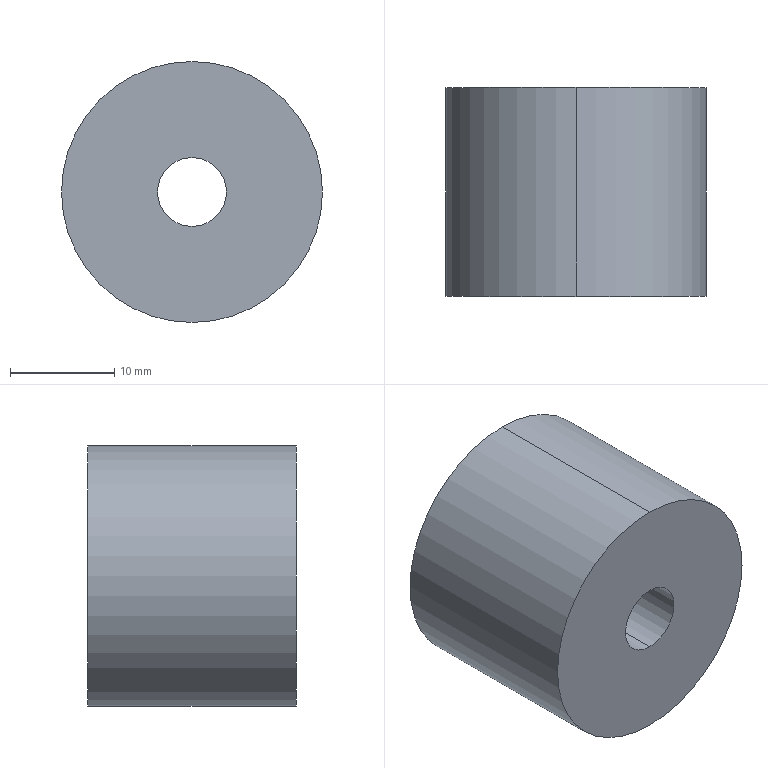Part | SolidWorks | features Extrusion 1, HoleWzd 1 | 1 solid | 9 faces | box 25 x 20 x 25 mm | volume 8476 mm3 | cylinder 6 | plane 3 | commonest cylinder face diameters 6.6 x2 11 x2 25 x2
STEP:
#1=CARTESIAN_POINT('',(0.,9.2,-5.5));
#2=VERTEX_POINT('',#1);
#3=CARTESIAN_POINT('',(0.,9.2,5.5));
#4=VERTEX_POINT('',#3);
#5=CARTESIAN_POINT('',(0.,9.2,0.));
#6=DIRECTION('',(0.,1.,0.));
#7=DIRECTION('',(0.,0.,1.));
#8=AXIS2_PLACEMENT_3D('',#5,#6,#7);
#9=CIRCLE('',#8,5.5);
#10=EDGE_CURVE('',#2,#4,#9,.T.);
#11=ORIENTED_EDGE('',*,*,#10,.F.);
#12=CARTESIAN_POINT('',(0.,20.,-5.5));
#13=VERTEX_POINT('',#12);
#14=CARTESIAN_POINT('',(0.,20.,-5.5));
#15=DIRECTION('',(0.,1.,0.));
#16=VECTOR('',#15,1000.);
#17=LINE('',#14,#16);
#18=EDGE_CURVE('',#2,#13,#17,.T.);
#19=ORIENTED_EDGE('',*,*,#18,.T.);
#20=CARTESIAN_POINT('',(0.,20.,5.5));
#21=VERTEX_POINT('',#20);
#22=CARTESIAN_POINT('',(0.,20.,0.));
#23=DIRECTION('',(0.,1.,0.));
#24=DIRECTION('',(0.,0.,1.));
#25=AXIS2_PLACEMENT_3D('',#22,#23,#24);
#26=CIRCLE('',#25,5.5);
#27=EDGE_CURVE('',#13,#21,#26,.T.);
#28=ORIENTED_EDGE('',*,*,#27,.T.);
#29=CARTESIAN_POINT('',(0.,20.,5.5));
#30=DIRECTION('',(0.,1.,0.));
#31=VECTOR('',#30,1000.);
#32=LINE('',#29,#31);
#33=EDGE_CURVE('',#4,#21,#32,.T.);
#34=ORIENTED_EDGE('',*,*,#33,.F.);
#35=EDGE_LOOP('',(#11,#19,#28,#34));
#36=FACE_OUTER_BOUND('',#35,.T.);
#37=CARTESIAN_POINT('',(0.,20.,0.));
#38=DIRECTION('',(0.,1.,0.));
#39=DIRECTION('',(0.,0.,1.));
#40=AXIS2_PLACEMENT_3D('',#37,#38,#39);
#41=CYLINDRICAL_SURFACE('',#40,5.5);
#42=ADVANCED_FACE('',(#36),#41,.F.);
#43=CARTESIAN_POINT('',(0.,0.,-3.3));
#44=VERTEX_POINT('',#43);
#45=CARTESIAN_POINT('',(0.,0.,3.3));
#46=VERTEX_POINT('',#45);
#47=CARTESIAN_POINT('',(0.,0.,0.));
#48=DIRECTION('',(0.,1.,0.));
#49=DIRECTION('',(0.,0.,1.));
#50=AXIS2_PLACEMENT_3D('',#47,#48,#49);
#51=CIRCLE('',#50,3.3);
#52=EDGE_CURVE('',#44,#46,#51,.T.);
#53=ORIENTED_EDGE('',*,*,#52,.F.);
#54=CARTESIAN_POINT('',(0.,9.2,-3.3));
#55=VERTEX_POINT('',#54);
#56=CARTESIAN_POINT('',(0.,20.,-3.3));
#57=DIRECTION('',(0.,1.,0.));
#58=VECTOR('',#57,1000.);
#59=LINE('',#56,#58);
#60=EDGE_CURVE('',#44,#55,#59,.T.);
#61=ORIENTED_EDGE('',*,*,#60,.T.);
#62=CARTESIAN_POINT('',(0.,9.2,3.3));
#63=VERTEX_POINT('',#62);
#64=CARTESIAN_POINT('',(0.,9.2,0.));
#65=DIRECTION('',(0.,1.,0.));
#66=DIRECTION('',(0.,0.,1.));
#67=AXIS2_PLACEMENT_3D('',#64,#65,#66);
#68=CIRCLE('',#67,3.3);
#69=EDGE_CURVE('',#55,#63,#68,.T.);
#70=ORIENTED_EDGE('',*,*,#69,.T.);
#71=CARTESIAN_POINT('',(0.,20.,3.3));
#72=DIRECTION('',(0.,1.,0.));
#73=VECTOR('',#72,1000.);
#74=LINE('',#71,#73);
#75=EDGE_CURVE('',#46,#63,#74,.T.);
#76=ORIENTED_EDGE('',*,*,#75,.F.);
#77=EDGE_LOOP('',(#53,#61,#70,#76));
#78=FACE_OUTER_BOUND('',#77,.T.);
#79=CARTESIAN_POINT('',(0.,20.,0.));
#80=DIRECTION('',(0.,1.,0.));
#81=DIRECTION('',(0.,0.,1.));
#82=AXIS2_PLACEMENT_3D('',#79,#80,#81);
#83=CYLINDRICAL_SURFACE('',#82,3.3);
#84=ADVANCED_FACE('',(#78),#83,.F.);
#85=CARTESIAN_POINT('',(0.,20.,12.5));
#86=VERTEX_POINT('',#85);
#87=CARTESIAN_POINT('',(0.,20.,-12.5));
#88=VERTEX_POINT('',#87);
#89=CARTESIAN_POINT('',(0.,20.,0.));
#90=DIRECTION('',(0.,1.,0.));
#91=DIRECTION('',(0.,0.,1.));
#92=AXIS2_PLACEMENT_3D('',#89,#90,#91);
#93=CIRCLE('',#92,12.5);
#94=EDGE_CURVE('',#86,#88,#93,.T.);
#95=ORIENTED_EDGE('',*,*,#94,.F.);
#96=CARTESIAN_POINT('',(0.,0.,12.5));
#97=VERTEX_POINT('',#96);
#98=CARTESIAN_POINT('',(0.,20.,12.5));
#99=DIRECTION('',(0.,-1.,0.));
#100=VECTOR('',#99,1000.);
#101=LINE('',#98,#100);
#102=EDGE_CURVE('',#86,#97,#101,.T.);
#103=ORIENTED_EDGE('',*,*,#102,.T.);
#104=CARTESIAN_POINT('',(0.,0.,-12.5));
#105=VERTEX_POINT('',#104);
#106=CARTESIAN_POINT('',(0.,0.,0.));
#107=DIRECTION('',(0.,1.,0.));
#108=DIRECTION('',(0.,0.,1.));
#109=AXIS2_PLACEMENT_3D('',#106,#107,#108);
#110=CIRCLE('',#109,12.5);
#111=EDGE_CURVE('',#97,#105,#110,.T.);
#112=ORIENTED_EDGE('',*,*,#111,.T.);
#113=CARTESIAN_POINT('',(0.,20.,-12.5));
#114=DIRECTION('',(0.,-1.,0.));
#115=VECTOR('',#114,1000.);
#116=LINE('',#113,#115);
#117=EDGE_CURVE('',#88,#105,#116,.T.);
#118=ORIENTED_EDGE('',*,*,#117,.F.);
#119=EDGE_LOOP('',(#95,#103,#112,#118));
#120=FACE_OUTER_BOUND('',#119,.T.);
#121=CARTESIAN_POINT('',(0.,20.,0.));
#122=DIRECTION('',(0.,-1.,0.));
#123=DIRECTION('',(0.,0.,-1.));
#124=AXIS2_PLACEMENT_3D('',#121,#122,#123);
#125=CYLINDRICAL_SURFACE('',#124,12.5);
#126=ADVANCED_FACE('',(#120),#125,.T.);
#127=ORIENTED_EDGE('',*,*,#102,.F.);
#128=CARTESIAN_POINT('',(0.,20.,0.));
#129=DIRECTION('',(0.,1.,0.));
#130=DIRECTION('',(0.,0.,1.));
#131=AXIS2_PLACEMENT_3D('',#128,#129,#130);
#132=CIRCLE('',#131,12.5);
#133=EDGE_CURVE('',#88,#86,#132,.T.);
#134=ORIENTED_EDGE('',*,*,#133,.F.);
#135=ORIENTED_EDGE('',*,*,#117,.T.);
#136=CARTESIAN_POINT('',(0.,0.,0.));
#137=DIRECTION('',(0.,1.,0.));
#138=DIRECTION('',(0.,0.,1.));
#139=AXIS2_PLACEMENT_3D('',#136,#137,#138);
#140=CIRCLE('',#139,12.5);
#141=EDGE_CURVE('',#105,#97,#140,.T.);
#142=ORIENTED_EDGE('',*,*,#141,.T.);
#143=EDGE_LOOP('',(#127,#134,#135,#142));
#144=FACE_OUTER_BOUND('',#143,.T.);
#145=CARTESIAN_POINT('',(0.,20.,0.));
#146=DIRECTION('',(0.,-1.,0.));
#147=DIRECTION('',(0.,0.,-1.));
#148=AXIS2_PLACEMENT_3D('',#145,#146,#147);
#149=CYLINDRICAL_SURFACE('',#148,12.5);
#150=ADVANCED_FACE('',(#144),#149,.T.);
#151=CARTESIAN_POINT('',(0.,20.,0.));
#152=DIRECTION('',(0.,1.,0.));
#153=DIRECTION('',(0.,0.,1.));
#154=AXIS2_PLACEMENT_3D('',#151,#152,#153);
#155=CIRCLE('',#154,5.5);
#156=EDGE_CURVE('',#21,#13,#155,.T.);
#157=ORIENTED_EDGE('',*,*,#156,.F.);
#158=ORIENTED_EDGE('',*,*,#27,.F.);
#159=EDGE_LOOP('',(#157,#158));
#160=FACE_BOUND('',#159,.T.);
#161=ORIENTED_EDGE('',*,*,#133,.T.);
#162=ORIENTED_EDGE('',*,*,#94,.T.);
#163=EDGE_LOOP('',(#161,#162));
#164=FACE_OUTER_BOUND('',#163,.T.);
#165=CARTESIAN_POINT('',(0.,20.,0.));
#166=DIRECTION('',(0.,1.,0.));
#167=DIRECTION('',(0.,0.,1.));
#168=AXIS2_PLACEMENT_3D('',#165,#166,#167);
#169=PLANE('',#168);
#170=ADVANCED_FACE('',(#160,#164),#169,.T.);
#171=CARTESIAN_POINT('',(0.,0.,0.));
#172=DIRECTION('',(0.,1.,0.));
#173=DIRECTION('',(0.,0.,1.));
#174=AXIS2_PLACEMENT_3D('',#171,#172,#173);
#175=CIRCLE('',#174,3.3);
#176=EDGE_CURVE('',#46,#44,#175,.T.);
#177=ORIENTED_EDGE('',*,*,#176,.T.);
#178=ORIENTED_EDGE('',*,*,#52,.T.);
#179=EDGE_LOOP('',(#177,#178));
#180=FACE_BOUND('',#179,.T.);
#181=ORIENTED_EDGE('',*,*,#141,.F.);
#182=ORIENTED_EDGE('',*,*,#111,.F.);
#183=EDGE_LOOP('',(#181,#182));
#184=FACE_OUTER_BOUND('',#183,.T.);
#185=CARTESIAN_POINT('',(0.,0.,0.));
#186=DIRECTION('',(0.,1.,0.));
#187=DIRECTION('',(0.,0.,1.));
#188=AXIS2_PLACEMENT_3D('',#185,#186,#187);
#189=PLANE('',#188);
#190=ADVANCED_FACE('',(#180,#184),#189,.F.);
#191=ORIENTED_EDGE('',*,*,#60,.F.);
#192=ORIENTED_EDGE('',*,*,#176,.F.);
#193=ORIENTED_EDGE('',*,*,#75,.T.);
#194=CARTESIAN_POINT('',(0.,9.2,0.));
#195=DIRECTION('',(0.,1.,0.));
#196=DIRECTION('',(0.,0.,1.));
#197=AXIS2_PLACEMENT_3D('',#194,#195,#196);
#198=CIRCLE('',#197,3.3);
#199=EDGE_CURVE('',#63,#55,#198,.T.);
#200=ORIENTED_EDGE('',*,*,#199,.T.);
#201=EDGE_LOOP('',(#191,#192,#193,#200));
#202=FACE_OUTER_BOUND('',#201,.T.);
#203=CARTESIAN_POINT('',(0.,20.,0.));
#204=DIRECTION('',(0.,1.,0.));
#205=DIRECTION('',(0.,0.,1.));
#206=AXIS2_PLACEMENT_3D('',#203,#204,#205);
#207=CYLINDRICAL_SURFACE('',#206,3.3);
#208=ADVANCED_FACE('',(#202),#207,.F.);
#209=ORIENTED_EDGE('',*,*,#199,.F.);
#210=ORIENTED_EDGE('',*,*,#69,.F.);
#211=EDGE_LOOP('',(#209,#210));
#212=FACE_BOUND('',#211,.T.);
#213=CARTESIAN_POINT('',(0.,9.2,0.));
#214=DIRECTION('',(0.,1.,0.));
#215=DIRECTION('',(0.,0.,1.));
#216=AXIS2_PLACEMENT_3D('',#213,#214,#215);
#217=CIRCLE('',#216,5.5);
#218=EDGE_CURVE('',#4,#2,#217,.T.);
#219=ORIENTED_EDGE('',*,*,#218,.T.);
#220=ORIENTED_EDGE('',*,*,#10,.T.);
#221=EDGE_LOOP('',(#219,#220));
#222=FACE_OUTER_BOUND('',#221,.T.);
#223=CARTESIAN_POINT('',(3.3,9.2,0.));
#224=DIRECTION('',(0.,-1.,0.));
#225=DIRECTION('',(0.,0.,-1.));
#226=AXIS2_PLACEMENT_3D('',#223,#224,#225);
#227=PLANE('',#226);
#228=ADVANCED_FACE('',(#212,#222),#227,.F.);
#229=ORIENTED_EDGE('',*,*,#18,.F.);
#230=ORIENTED_EDGE('',*,*,#218,.F.);
#231=ORIENTED_EDGE('',*,*,#33,.T.);
#232=ORIENTED_EDGE('',*,*,#156,.T.);
#233=EDGE_LOOP('',(#229,#230,#231,#232));
#234=FACE_OUTER_BOUND('',#233,.T.);
#235=CARTESIAN_POINT('',(0.,20.,0.));
#236=DIRECTION('',(0.,1.,0.));
#237=DIRECTION('',(0.,0.,1.));
#238=AXIS2_PLACEMENT_3D('',#235,#236,#237);
#239=CYLINDRICAL_SURFACE('',#238,5.5);
#240=ADVANCED_FACE('',(#234),#239,.F.);
#241=CLOSED_SHELL('',(#42,#84,#126,#150,#170,#190,#208,#228,#240));
#242=MANIFOLD_SOLID_BREP('',#241);
#243=CARTESIAN_POINT('',(0.,0.,0.));
#244=DIRECTION('',(0.,0.,1.));
#245=DIRECTION('',(1.,0.,0.));
#246=AXIS2_PLACEMENT_3D('',#243,#244,#245);
#247=(LENGTH_UNIT()NAMED_UNIT(*)SI_UNIT(.MILLI.,.METRE.));
#248=UNCERTAINTY_MEASURE_WITH_UNIT(LENGTH_MEASURE(0.00001),#247,'','');
#249=(NAMED_UNIT(*)PLANE_ANGLE_UNIT()SI_UNIT($,.RADIAN.));
#250=(NAMED_UNIT(*)SI_UNIT($,.STERADIAN.)SOLID_ANGLE_UNIT());
#251=(GEOMETRIC_REPRESENTATION_CONTEXT(3)GLOBAL_UNCERTAINTY_ASSIGNED_CONTEXT((#248))GLOBAL_UNIT_ASSIGNED_CONTEXT((#247,#249,#250))REPRESENTATION_CONTEXT('',''));
#252=ADVANCED_BREP_SHAPE_REPRESENTATION('',(#242,#246),#251);